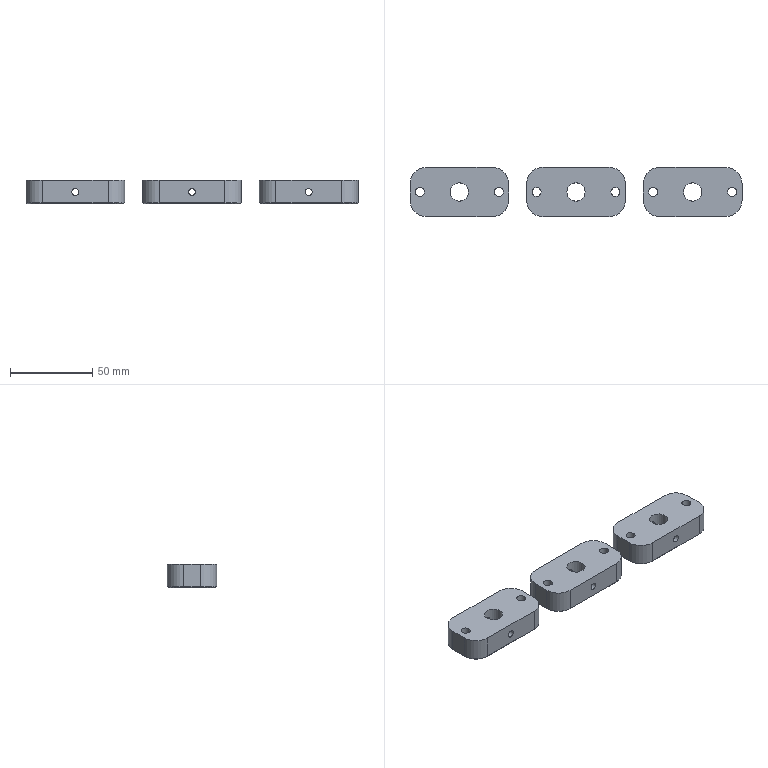Part | 3 solids | 87 faces | box 202 x 30 x 14 mm | volume 63770 mm3 | plane 36 | cylinder 33 | cone 18 | commonest cylinder face diameters 20 x12 4.2 x6 5.5 x6 9 x6 11.06 x3